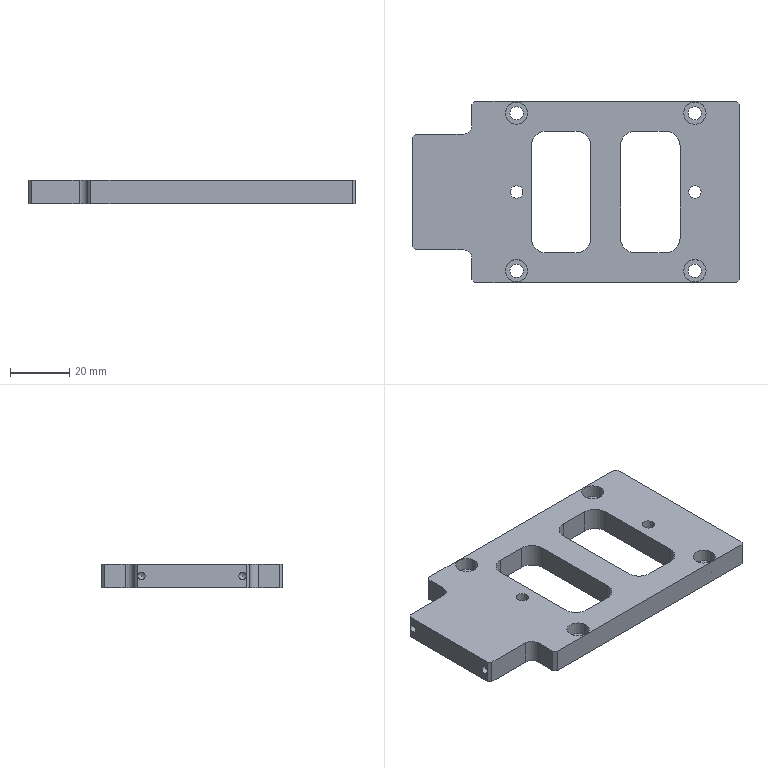CAM job | NX | 3-axis milling, drilling | part box 110 x 61 x 8 mm | stock box 115 x 66 x 10 mm
Tools:
number,name,description,diameter,corner_radius,flute_length,length,flutes
4,D4,平底铣刀-粗,4.0,0.0,25.0,75.0,2
9,D10,平底铣刀-粗,10.0,0.0,35.0,75.0,2
7,D6-J,平底铣刀-精,6.0,0.0,25.0,75.0,2
1,D80R0.8飞刀,圆鼻刀-粗,80.0,0.8,50.0,75.0,2
1,D80R0.8飞刀-J,圆鼻刀-精,80.0,0.8,50.0,75.0,2
2,D6倒角刀,倒角刀,6.0,0.0,3.0,25.0,2
22,M5X0.8,丝锥,4.2,0.0,35.0,50.0,2
11,ZT4.5,钻头,4.5,0.0,35.0,50.0,2
14,钻头4.2,Twist Drill 4.2 mm,4.2,0.0,41.0,41.738,2
Operations:
program,operation,operation_type,tool,method,geometry_group,spindle_rpm,surface_speed,feed_per_tooth,feed_cut,feed_plunge,cut_length_mm,path_length_mm,cut_time_min,machine_time_min
B,底壁铣飞面一刀开粗_COPY,VolumeBased25DMillingOperation,D80R0.8飞刀,分层开粗-切深K-步距G,W-B,2800.0,703.696,0.5357,3000.0,100.0,872.776,1549.735,0.2909,0.3586
B,底壁铣飞面一刀精光_COPY,VolumeBased25DMillingOperation,D80R0.8飞刀-J,侧刃精光-切深K-步距G,W-B,4000.0,1005.28,0.125,1000.0,100.0,217.998,253.998,0.218,0.2216
B,钻倒角_1,Operation,D6倒角刀,METHOD,W-B,8000.0,150.796,0.0625,1000.0,0.0,11.4,125.875,0.0114,0.0228
B,钻倒角_2,Operation,D6倒角刀,METHOD,W-B,8000.0,150.796,0.0625,1000.0,0.0,22.2,259.645,0.0222,0.0459
B,平面去毛刺6X45L_COPY,SurfaceContour,D6倒角刀,爬面_倒角-切深0-步距G,W-B,6500.0,122.519,0.1154,1500.0,100.0,636.101,1087.001,0.4241,0.4692
A,顶面,FaceMilling,D80R0.8飞刀,侧刃精光-切深K-步距G,W-A,4000.0,1005.31,0.125,1000.0,100.0,204.0,240.0,0.204,0.2076
A,型腔铣开粗-中_COPY,CavityMilling,D10,分层开粗-切深K-步距G,W-A,8000.0,251.32,0.25,4000.0,100.0,14109.856,14572.703,3.527,3.598
A,框开粗_1,VolumeBased25DMillingOperation,D10,METHOD,W-A,6000.0,188.0,0.25,4000.0,80.0,3088.655,3212.66,0.7722,0.7846
A,打点-深0.8,Operation,D6倒角刀,NONE,W-A,8000.0,150.796,0.0312,500.0,90.0,10.8,232.684,0.0216,0.0438
A,通孔-M5螺纹底孔,Operation,钻头4.2,NONE,W-A,3000.0,39.584,0.0583,350.0,90.0,32.524,166.056,0.0929,0.1063
A,沉头孔-钻孔0段,Operation,ZT4.5,NONE,W-A,2800.0,39.584,0.0179,100.0,90.0,49.408,307.843,0.4941,0.5199
A,铣孔开粗D4_1,CylinderMilling,D4,NONE,W-A,8000.0,100.531,0.075,1200.0,100.0,739.814,1081.414,0.6165,0.6507
A,铣孔精光D4_1,CylinderMilling,D4,精光步距切深关,W-A,8000.0,100.531,0.0312,500.0,100.0,113.064,454.664,0.2261,0.2603
A,框精_1,VolumeBased25DMillingOperation,D6-J,METHOD,W-A,6000.0,113.0,0.0833,1000.0,100.0,200.815,342.715,0.2008,0.215
A,外形侧面,ZLevelMilling,D6-J,METHOD,W-A,9000.0,84.823,0.1389,2500.0,80.0,461.178,600.867,0.1848,0.1988
A,仅选体,SurfaceContour,D6倒角刀,METHOD,W-A,8000.0,150.796,0.1875,3000.0,100.0,581.994,737.348,0.194,0.2095
A,铣倒角_1,PlanarMilling,D6倒角刀,METHOD,W-A,8000.0,150.796,0.0312,500.0,100.0,36.041,178.057,0.0721,0.0863
A,铣倒角_2,PlanarMilling,D6倒角刀,NONE,W-A,8000.0,150.796,0.0312,500.0,100.0,129.588,446.341,0.2592,0.2909
A,通孔-攻牙M5,Operation,M5X0.8,METHOD,W-A,500.0,6.597,0.0008,0.8,90.0,25.0,151.008,31.25,31.263
A,外形半精_2,VolumeBased25DMillingOperation,D6-J,METHOD,W-A,8000.0,251.327,0.0625,1000.0,100.0,359.676,414.876,0.3597,0.3652